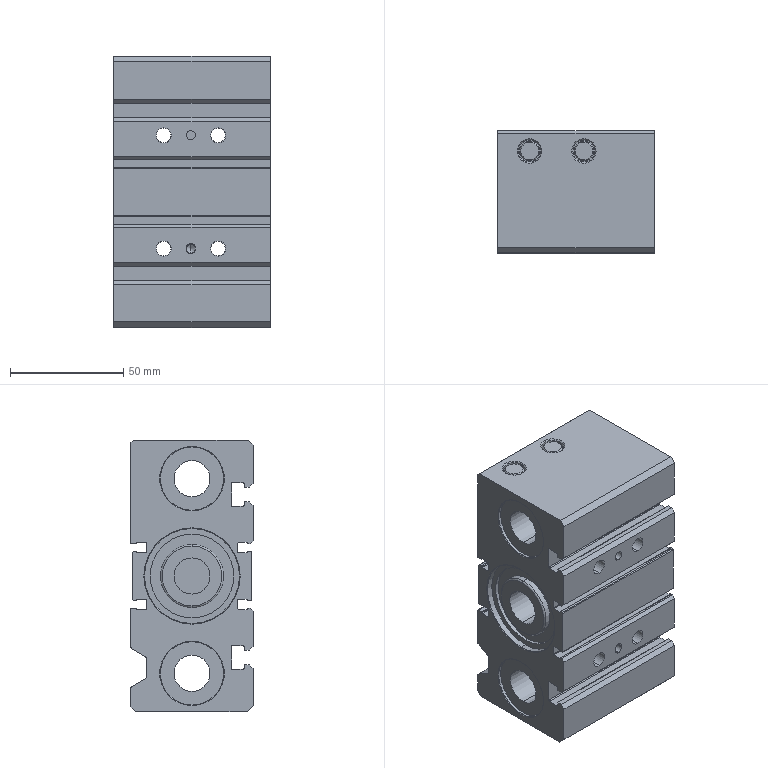Part | SolidWorks | features BaseBody 1 | 1 solid | 292 faces | box 69 x 54 x 120 mm | volume 283618 mm3 | cylinder 132 | plane 96 | cone 60 | torus 4 | commonest cylinder face diameters 0.8 x28 6.647 x16 4 x14 0.4 x12 6.5 x8 11 x8